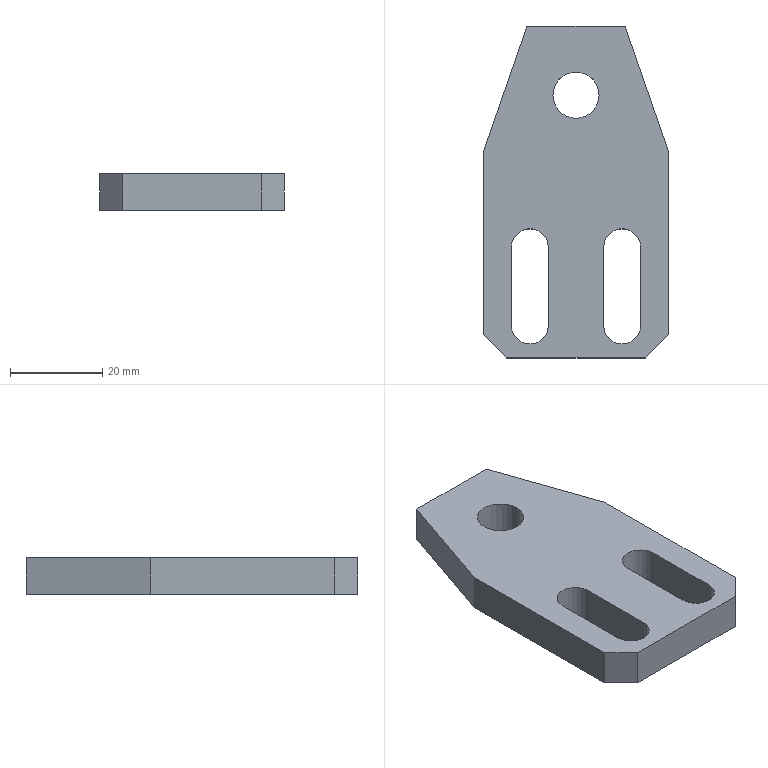Part | SolidWorks | features Chamfer 1, Extrusion 1 | 1 solid | 20 faces | box 40 x 72 x 8 mm | volume 17211 mm3 | plane 14 | cylinder 6 | commonest cylinder face diameters 8 x4 10 x2
STEP:
#1=CARTESIAN_POINT('',(-5.,57.,8.));
#2=VERTEX_POINT('',#1);
#3=CARTESIAN_POINT('',(5.,57.,8.));
#4=VERTEX_POINT('',#3);
#5=CARTESIAN_POINT('',(0.,57.,8.));
#6=DIRECTION('',(0.,0.,1.));
#7=DIRECTION('',(1.,0.,0.));
#8=AXIS2_PLACEMENT_3D('',#5,#6,#7);
#9=CIRCLE('',#8,5.);
#10=EDGE_CURVE('',#2,#4,#9,.T.);
#11=ORIENTED_EDGE('',*,*,#10,.T.);
#12=CARTESIAN_POINT('',(5.,57.,0.));
#13=VERTEX_POINT('',#12);
#14=CARTESIAN_POINT('',(5.,57.,8.));
#15=DIRECTION('',(0.,0.,-1.));
#16=VECTOR('',#15,1000.);
#17=LINE('',#14,#16);
#18=EDGE_CURVE('',#4,#13,#17,.T.);
#19=ORIENTED_EDGE('',*,*,#18,.T.);
#20=CARTESIAN_POINT('',(-5.,57.,0.));
#21=VERTEX_POINT('',#20);
#22=CARTESIAN_POINT('',(0.,57.,0.));
#23=DIRECTION('',(0.,0.,1.));
#24=DIRECTION('',(1.,0.,0.));
#25=AXIS2_PLACEMENT_3D('',#22,#23,#24);
#26=CIRCLE('',#25,5.);
#27=EDGE_CURVE('',#21,#13,#26,.T.);
#28=ORIENTED_EDGE('',*,*,#27,.F.);
#29=CARTESIAN_POINT('',(-5.,57.,8.));
#30=DIRECTION('',(0.,0.,-1.));
#31=VECTOR('',#30,1000.);
#32=LINE('',#29,#31);
#33=EDGE_CURVE('',#2,#21,#32,.T.);
#34=ORIENTED_EDGE('',*,*,#33,.F.);
#35=EDGE_LOOP('',(#11,#19,#28,#34));
#36=FACE_OUTER_BOUND('',#35,.T.);
#37=CARTESIAN_POINT('',(0.,57.,8.));
#38=DIRECTION('',(0.,0.,-1.));
#39=DIRECTION('',(-1.,0.,0.));
#40=AXIS2_PLACEMENT_3D('',#37,#38,#39);
#41=CYLINDRICAL_SURFACE('',#40,5.);
#42=ADVANCED_FACE('',(#36),#41,.F.);
#43=CARTESIAN_POINT('',(14.,7.,0.));
#44=VERTEX_POINT('',#43);
#45=CARTESIAN_POINT('',(14.,24.,0.));
#46=VERTEX_POINT('',#45);
#47=CARTESIAN_POINT('',(14.,0.,0.));
#48=DIRECTION('',(0.,1.,0.));
#49=VECTOR('',#48,1000.);
#50=LINE('',#47,#49);
#51=EDGE_CURVE('',#44,#46,#50,.T.);
#52=ORIENTED_EDGE('',*,*,#51,.F.);
#53=CARTESIAN_POINT('',(14.,7.,8.));
#54=VERTEX_POINT('',#53);
#55=CARTESIAN_POINT('',(14.,7.,8.));
#56=DIRECTION('',(0.,0.,-1.));
#57=VECTOR('',#56,1000.);
#58=LINE('',#55,#57);
#59=EDGE_CURVE('',#54,#44,#58,.T.);
#60=ORIENTED_EDGE('',*,*,#59,.F.);
#61=CARTESIAN_POINT('',(14.,24.,8.));
#62=VERTEX_POINT('',#61);
#63=CARTESIAN_POINT('',(14.,0.,8.));
#64=DIRECTION('',(0.,1.,0.));
#65=VECTOR('',#64,1000.);
#66=LINE('',#63,#65);
#67=EDGE_CURVE('',#54,#62,#66,.T.);
#68=ORIENTED_EDGE('',*,*,#67,.T.);
#69=CARTESIAN_POINT('',(14.,24.,8.));
#70=DIRECTION('',(0.,0.,-1.));
#71=VECTOR('',#70,1000.);
#72=LINE('',#69,#71);
#73=EDGE_CURVE('',#62,#46,#72,.T.);
#74=ORIENTED_EDGE('',*,*,#73,.T.);
#75=EDGE_LOOP('',(#52,#60,#68,#74));
#76=FACE_OUTER_BOUND('',#75,.T.);
#77=CARTESIAN_POINT('',(14.,0.,8.));
#78=DIRECTION('',(-1.,0.,0.));
#79=DIRECTION('',(0.,-1.,0.));
#80=AXIS2_PLACEMENT_3D('',#77,#78,#79);
#81=PLANE('',#80);
#82=ADVANCED_FACE('',(#76),#81,.T.);
#83=CARTESIAN_POINT('',(6.,7.,0.));
#84=VERTEX_POINT('',#83);
#85=CARTESIAN_POINT('',(10.,7.,0.));
#86=DIRECTION('',(0.,0.,-1.));
#87=DIRECTION('',(1.,0.,0.));
#88=AXIS2_PLACEMENT_3D('',#85,#86,#87);
#89=CIRCLE('',#88,4.);
#90=EDGE_CURVE('',#44,#84,#89,.T.);
#91=ORIENTED_EDGE('',*,*,#90,.T.);
#92=CARTESIAN_POINT('',(6.,7.,8.));
#93=VERTEX_POINT('',#92);
#94=CARTESIAN_POINT('',(6.,7.,8.));
#95=DIRECTION('',(0.,0.,-1.));
#96=VECTOR('',#95,1000.);
#97=LINE('',#94,#96);
#98=EDGE_CURVE('',#93,#84,#97,.T.);
#99=ORIENTED_EDGE('',*,*,#98,.F.);
#100=CARTESIAN_POINT('',(10.,7.,8.));
#101=DIRECTION('',(0.,0.,-1.));
#102=DIRECTION('',(1.,0.,0.));
#103=AXIS2_PLACEMENT_3D('',#100,#101,#102);
#104=CIRCLE('',#103,4.);
#105=EDGE_CURVE('',#54,#93,#104,.T.);
#106=ORIENTED_EDGE('',*,*,#105,.F.);
#107=ORIENTED_EDGE('',*,*,#59,.T.);
#108=EDGE_LOOP('',(#91,#99,#106,#107));
#109=FACE_OUTER_BOUND('',#108,.T.);
#110=CARTESIAN_POINT('',(10.,7.,8.));
#111=DIRECTION('',(0.,0.,-1.));
#112=DIRECTION('',(-1.,0.,0.));
#113=AXIS2_PLACEMENT_3D('',#110,#111,#112);
#114=CYLINDRICAL_SURFACE('',#113,4.);
#115=ADVANCED_FACE('',(#109),#114,.F.);
#116=CARTESIAN_POINT('',(6.,24.,0.));
#117=VERTEX_POINT('',#116);
#118=CARTESIAN_POINT('',(6.,0.,0.));
#119=DIRECTION('',(0.,1.,0.));
#120=VECTOR('',#119,1000.);
#121=LINE('',#118,#120);
#122=EDGE_CURVE('',#84,#117,#121,.T.);
#123=ORIENTED_EDGE('',*,*,#122,.T.);
#124=CARTESIAN_POINT('',(6.,24.,8.));
#125=VERTEX_POINT('',#124);
#126=CARTESIAN_POINT('',(6.,24.,8.));
#127=DIRECTION('',(0.,0.,-1.));
#128=VECTOR('',#127,1000.);
#129=LINE('',#126,#128);
#130=EDGE_CURVE('',#125,#117,#129,.T.);
#131=ORIENTED_EDGE('',*,*,#130,.F.);
#132=CARTESIAN_POINT('',(6.,0.,8.));
#133=DIRECTION('',(0.,1.,0.));
#134=VECTOR('',#133,1000.);
#135=LINE('',#132,#134);
#136=EDGE_CURVE('',#93,#125,#135,.T.);
#137=ORIENTED_EDGE('',*,*,#136,.F.);
#138=ORIENTED_EDGE('',*,*,#98,.T.);
#139=EDGE_LOOP('',(#123,#131,#137,#138));
#140=FACE_OUTER_BOUND('',#139,.T.);
#141=CARTESIAN_POINT('',(6.,0.,8.));
#142=DIRECTION('',(-1.,0.,0.));
#143=DIRECTION('',(0.,0.,1.));
#144=AXIS2_PLACEMENT_3D('',#141,#142,#143);
#145=PLANE('',#144);
#146=ADVANCED_FACE('',(#140),#145,.F.);
#147=CARTESIAN_POINT('',(-15.,0.,8.));
#148=VERTEX_POINT('',#147);
#149=CARTESIAN_POINT('',(15.,0.,8.));
#150=VERTEX_POINT('',#149);
#151=CARTESIAN_POINT('',(0.,0.,8.));
#152=DIRECTION('',(1.,0.,0.));
#153=VECTOR('',#152,1000.);
#154=LINE('',#151,#153);
#155=EDGE_CURVE('',#148,#150,#154,.T.);
#156=ORIENTED_EDGE('',*,*,#155,.F.);
#157=CARTESIAN_POINT('',(-15.,0.,0.));
#158=VERTEX_POINT('',#157);
#159=CARTESIAN_POINT('',(-15.,0.,8.));
#160=DIRECTION('',(0.,0.,-1.));
#161=VECTOR('',#160,1000.);
#162=LINE('',#159,#161);
#163=EDGE_CURVE('',#148,#158,#162,.T.);
#164=ORIENTED_EDGE('',*,*,#163,.T.);
#165=CARTESIAN_POINT('',(15.,0.,0.));
#166=VERTEX_POINT('',#165);
#167=CARTESIAN_POINT('',(0.,0.,0.));
#168=DIRECTION('',(1.,0.,0.));
#169=VECTOR('',#168,1000.);
#170=LINE('',#167,#169);
#171=EDGE_CURVE('',#158,#166,#170,.T.);
#172=ORIENTED_EDGE('',*,*,#171,.T.);
#173=CARTESIAN_POINT('',(15.,0.,8.));
#174=DIRECTION('',(0.,0.,1.));
#175=VECTOR('',#174,1000.);
#176=LINE('',#173,#175);
#177=EDGE_CURVE('',#166,#150,#176,.T.);
#178=ORIENTED_EDGE('',*,*,#177,.T.);
#179=EDGE_LOOP('',(#156,#164,#172,#178));
#180=FACE_OUTER_BOUND('',#179,.T.);
#181=CARTESIAN_POINT('',(0.,0.,8.));
#182=DIRECTION('',(0.,1.,0.));
#183=DIRECTION('',(0.,0.,1.));
#184=AXIS2_PLACEMENT_3D('',#181,#182,#183);
#185=PLANE('',#184);
#186=ADVANCED_FACE('',(#180),#185,.F.);
#187=CARTESIAN_POINT('',(20.,5.,8.));
#188=VERTEX_POINT('',#187);
#189=CARTESIAN_POINT('',(20.,45.,8.));
#190=VERTEX_POINT('',#189);
#191=CARTESIAN_POINT('',(20.,0.,8.));
#192=DIRECTION('',(0.,1.,0.));
#193=VECTOR('',#192,1000.);
#194=LINE('',#191,#193);
#195=EDGE_CURVE('',#188,#190,#194,.T.);
#196=ORIENTED_EDGE('',*,*,#195,.F.);
#197=CARTESIAN_POINT('',(20.,5.,0.));
#198=VERTEX_POINT('',#197);
#199=CARTESIAN_POINT('',(20.,5.,8.));
#200=DIRECTION('',(0.,0.,-1.));
#201=VECTOR('',#200,1000.);
#202=LINE('',#199,#201);
#203=EDGE_CURVE('',#188,#198,#202,.T.);
#204=ORIENTED_EDGE('',*,*,#203,.T.);
#205=CARTESIAN_POINT('',(20.,45.,0.));
#206=VERTEX_POINT('',#205);
#207=CARTESIAN_POINT('',(20.,0.,0.));
#208=DIRECTION('',(0.,1.,0.));
#209=VECTOR('',#208,1000.);
#210=LINE('',#207,#209);
#211=EDGE_CURVE('',#198,#206,#210,.T.);
#212=ORIENTED_EDGE('',*,*,#211,.T.);
#213=CARTESIAN_POINT('',(20.,45.,8.));
#214=DIRECTION('',(0.,0.,-1.));
#215=VECTOR('',#214,1000.);
#216=LINE('',#213,#215);
#217=EDGE_CURVE('',#190,#206,#216,.T.);
#218=ORIENTED_EDGE('',*,*,#217,.F.);
#219=EDGE_LOOP('',(#196,#204,#212,#218));
#220=FACE_OUTER_BOUND('',#219,.T.);
#221=CARTESIAN_POINT('',(20.,0.,8.));
#222=DIRECTION('',(-1.,0.,0.));
#223=DIRECTION('',(0.,-1.,0.));
#224=AXIS2_PLACEMENT_3D('',#221,#222,#223);
#225=PLANE('',#224);
#226=ADVANCED_FACE('',(#220),#225,.F.);
#227=CARTESIAN_POINT('',(10.645,72.,0.));
#228=VERTEX_POINT('',#227);
#229=CARTESIAN_POINT('',(31.777,11.01,0.));
#230=DIRECTION('',(-0.3274,0.9449,0.));
#231=VECTOR('',#230,1000.);
#232=LINE('',#229,#231);
#233=EDGE_CURVE('',#206,#228,#232,.T.);
#234=ORIENTED_EDGE('',*,*,#233,.T.);
#235=CARTESIAN_POINT('',(10.645,72.,8.));
#236=VERTEX_POINT('',#235);
#237=CARTESIAN_POINT('',(10.645,72.,8.));
#238=DIRECTION('',(0.,0.,-1.));
#239=VECTOR('',#238,1000.);
#240=LINE('',#237,#239);
#241=EDGE_CURVE('',#236,#228,#240,.T.);
#242=ORIENTED_EDGE('',*,*,#241,.F.);
#243=CARTESIAN_POINT('',(31.777,11.01,8.));
#244=DIRECTION('',(-0.3274,0.9449,0.));
#245=VECTOR('',#244,1000.);
#246=LINE('',#243,#245);
#247=EDGE_CURVE('',#190,#236,#246,.T.);
#248=ORIENTED_EDGE('',*,*,#247,.F.);
#249=ORIENTED_EDGE('',*,*,#217,.T.);
#250=EDGE_LOOP('',(#234,#242,#248,#249));
#251=FACE_OUTER_BOUND('',#250,.T.);
#252=CARTESIAN_POINT('',(31.777,11.01,8.));
#253=DIRECTION('',(-0.9449,-0.3274,0.));
#254=DIRECTION('',(0.3274,-0.9449,0.));
#255=AXIS2_PLACEMENT_3D('',#252,#253,#254);
#256=PLANE('',#255);
#257=ADVANCED_FACE('',(#251),#256,.F.);
#258=CARTESIAN_POINT('',(-10.645,72.,0.));
#259=VERTEX_POINT('',#258);
#260=CARTESIAN_POINT('',(0.,72.,0.));
#261=DIRECTION('',(-1.,0.,0.));
#262=VECTOR('',#261,1000.);
#263=LINE('',#260,#262);
#264=EDGE_CURVE('',#228,#259,#263,.T.);
#265=ORIENTED_EDGE('',*,*,#264,.T.);
#266=CARTESIAN_POINT('',(-10.645,72.,8.));
#267=VERTEX_POINT('',#266);
#268=CARTESIAN_POINT('',(-10.645,72.,8.));
#269=DIRECTION('',(0.,0.,-1.));
#270=VECTOR('',#269,1000.);
#271=LINE('',#268,#270);
#272=EDGE_CURVE('',#267,#259,#271,.T.);
#273=ORIENTED_EDGE('',*,*,#272,.F.);
#274=CARTESIAN_POINT('',(0.,72.,8.));
#275=DIRECTION('',(-1.,0.,0.));
#276=VECTOR('',#275,1000.);
#277=LINE('',#274,#276);
#278=EDGE_CURVE('',#236,#267,#277,.T.);
#279=ORIENTED_EDGE('',*,*,#278,.F.);
#280=ORIENTED_EDGE('',*,*,#241,.T.);
#281=EDGE_LOOP('',(#265,#273,#279,#280));
#282=FACE_OUTER_BOUND('',#281,.T.);
#283=CARTESIAN_POINT('',(0.,72.,8.));
#284=DIRECTION('',(0.,-1.,0.));
#285=DIRECTION('',(0.,0.,-1.));
#286=AXIS2_PLACEMENT_3D('',#283,#284,#285);
#287=PLANE('',#286);
#288=ADVANCED_FACE('',(#282),#287,.F.);
#289=CARTESIAN_POINT('',(-20.,45.,0.));
#290=VERTEX_POINT('',#289);
#291=CARTESIAN_POINT('',(-31.777,11.01,0.));
#292=DIRECTION('',(-0.3274,-0.9449,0.));
#293=VECTOR('',#292,1000.);
#294=LINE('',#291,#293);
#295=EDGE_CURVE('',#259,#290,#294,.T.);
#296=ORIENTED_EDGE('',*,*,#295,.T.);
#297=CARTESIAN_POINT('',(-20.,45.,8.));
#298=VERTEX_POINT('',#297);
#299=CARTESIAN_POINT('',(-20.,45.,8.));
#300=DIRECTION('',(0.,0.,-1.));
#301=VECTOR('',#300,1000.);
#302=LINE('',#299,#301);
#303=EDGE_CURVE('',#298,#290,#302,.T.);
#304=ORIENTED_EDGE('',*,*,#303,.F.);
#305=CARTESIAN_POINT('',(-31.777,11.01,8.));
#306=DIRECTION('',(-0.3274,-0.9449,0.));
#307=VECTOR('',#306,1000.);
#308=LINE('',#305,#307);
#309=EDGE_CURVE('',#267,#298,#308,.T.);
#310=ORIENTED_EDGE('',*,*,#309,.F.);
#311=ORIENTED_EDGE('',*,*,#272,.T.);
#312=EDGE_LOOP('',(#296,#304,#310,#311));
#313=FACE_OUTER_BOUND('',#312,.T.);
#314=CARTESIAN_POINT('',(-31.777,11.01,8.));
#315=DIRECTION('',(0.9449,-0.3274,0.));
#316=DIRECTION('',(0.3274,0.9449,0.));
#317=AXIS2_PLACEMENT_3D('',#314,#315,#316);
#318=PLANE('',#317);
#319=ADVANCED_FACE('',(#313),#318,.F.);
#320=CARTESIAN_POINT('',(-6.,24.,0.));
#321=VERTEX_POINT('',#320);
#322=CARTESIAN_POINT('',(-14.,24.,0.));
#323=VERTEX_POINT('',#322);
#324=CARTESIAN_POINT('',(-10.,24.,0.));
#325=DIRECTION('',(0.,0.,1.));
#326=DIRECTION('',(1.,0.,0.));
#327=AXIS2_PLACEMENT_3D('',#324,#325,#326);
#328=CIRCLE('',#327,4.);
#329=EDGE_CURVE('',#321,#323,#328,.T.);
#330=ORIENTED_EDGE('',*,*,#329,.F.);
#331=CARTESIAN_POINT('',(-6.,24.,8.));
#332=VERTEX_POINT('',#331);
#333=CARTESIAN_POINT('',(-6.,24.,8.));
#334=DIRECTION('',(0.,0.,-1.));
#335=VECTOR('',#334,1000.);
#336=LINE('',#333,#335);
#337=EDGE_CURVE('',#332,#321,#336,.T.);
#338=ORIENTED_EDGE('',*,*,#337,.F.);
#339=CARTESIAN_POINT('',(-14.,24.,8.));
#340=VERTEX_POINT('',#339);
#341=CARTESIAN_POINT('',(-10.,24.,8.));
#342=DIRECTION('',(0.,0.,1.));
#343=DIRECTION('',(1.,0.,0.));
#344=AXIS2_PLACEMENT_3D('',#341,#342,#343);
#345=CIRCLE('',#344,4.);
#346=EDGE_CURVE('',#332,#340,#345,.T.);
#347=ORIENTED_EDGE('',*,*,#346,.T.);
#348=CARTESIAN_POINT('',(-14.,24.,8.));
#349=DIRECTION('',(0.,0.,-1.));
#350=VECTOR('',#349,1000.);
#351=LINE('',#348,#350);
#352=EDGE_CURVE('',#340,#323,#351,.T.);
#353=ORIENTED_EDGE('',*,*,#352,.T.);
#354=EDGE_LOOP('',(#330,#338,#347,#353));
#355=FACE_OUTER_BOUND('',#354,.T.);
#356=CARTESIAN_POINT('',(-10.,24.,8.));
#357=DIRECTION('',(0.,0.,-1.));
#358=DIRECTION('',(-1.,0.,0.));
#359=AXIS2_PLACEMENT_3D('',#356,#357,#358);
#360=CYLINDRICAL_SURFACE('',#359,4.);
#361=ADVANCED_FACE('',(#355),#360,.F.);
#362=CARTESIAN_POINT('',(-6.,7.,0.));
#363=VERTEX_POINT('',#362);
#364=CARTESIAN_POINT('',(-6.,0.,0.));
#365=DIRECTION('',(0.,1.,0.));
#366=VECTOR('',#365,1000.);
#367=LINE('',#364,#366);
#368=EDGE_CURVE('',#363,#321,#367,.T.);
#369=ORIENTED_EDGE('',*,*,#368,.F.);
#370=CARTESIAN_POINT('',(-6.,7.,8.));
#371=VERTEX_POINT('',#370);
#372=CARTESIAN_POINT('',(-6.,7.,8.));
#373=DIRECTION('',(0.,0.,-1.));
#374=VECTOR('',#373,1000.);
#375=LINE('',#372,#374);
#376=EDGE_CURVE('',#371,#363,#375,.T.);
#377=ORIENTED_EDGE('',*,*,#376,.F.);
#378=CARTESIAN_POINT('',(-6.,0.,8.));
#379=DIRECTION('',(0.,1.,0.));
#380=VECTOR('',#379,1000.);
#381=LINE('',#378,#380);
#382=EDGE_CURVE('',#371,#332,#381,.T.);
#383=ORIENTED_EDGE('',*,*,#382,.T.);
#384=ORIENTED_EDGE('',*,*,#337,.T.);
#385=EDGE_LOOP('',(#369,#377,#383,#384));
#386=FACE_OUTER_BOUND('',#385,.T.);
#387=CARTESIAN_POINT('',(-6.,0.,8.));
#388=DIRECTION('',(-1.,0.,0.));
#389=DIRECTION('',(0.,0.,1.));
#390=AXIS2_PLACEMENT_3D('',#387,#388,#389);
#391=PLANE('',#390);
#392=ADVANCED_FACE('',(#386),#391,.T.);
#393=CARTESIAN_POINT('',(-14.,7.,0.));
#394=VERTEX_POINT('',#393);
#395=CARTESIAN_POINT('',(-10.,7.,0.));
#396=DIRECTION('',(0.,0.,1.));
#397=DIRECTION('',(1.,0.,0.));
#398=AXIS2_PLACEMENT_3D('',#395,#396,#397);
#399=CIRCLE('',#398,4.);
#400=EDGE_CURVE('',#394,#363,#399,.T.);
#401=ORIENTED_EDGE('',*,*,#400,.F.);
#402=CARTESIAN_POINT('',(-14.,7.,8.));
#403=VERTEX_POINT('',#402);
#404=CARTESIAN_POINT('',(-14.,7.,8.));
#405=DIRECTION('',(0.,0.,-1.));
#406=VECTOR('',#405,1000.);
#407=LINE('',#404,#406);
#408=EDGE_CURVE('',#403,#394,#407,.T.);
#409=ORIENTED_EDGE('',*,*,#408,.F.);
#410=CARTESIAN_POINT('',(-10.,7.,8.));
#411=DIRECTION('',(0.,0.,1.));
#412=DIRECTION('',(1.,0.,0.));
#413=AXIS2_PLACEMENT_3D('',#410,#411,#412);
#414=CIRCLE('',#413,4.);
#415=EDGE_CURVE('',#403,#371,#414,.T.);
#416=ORIENTED_EDGE('',*,*,#415,.T.);
#417=ORIENTED_EDGE('',*,*,#376,.T.);
#418=EDGE_LOOP('',(#401,#409,#416,#417));
#419=FACE_OUTER_BOUND('',#418,.T.);
#420=CARTESIAN_POINT('',(-10.,7.,8.));
#421=DIRECTION('',(0.,0.,-1.));
#422=DIRECTION('',(-1.,0.,0.));
#423=AXIS2_PLACEMENT_3D('',#420,#421,#422);
#424=CYLINDRICAL_SURFACE('',#423,4.);
#425=ADVANCED_FACE('',(#419),#424,.F.);
#426=CARTESIAN_POINT('',(-20.,5.,0.));
#427=VERTEX_POINT('',#426);
#428=CARTESIAN_POINT('',(-20.,0.,0.));
#429=DIRECTION('',(0.,-1.,0.));
#430=VECTOR('',#429,1000.);
#431=LINE('',#428,#430);
#432=EDGE_CURVE('',#290,#427,#431,.T.);
#433=ORIENTED_EDGE('',*,*,#432,.T.);
#434=CARTESIAN_POINT('',(-20.,5.,8.));
#435=VERTEX_POINT('',#434);
#436=CARTESIAN_POINT('',(-20.,5.,8.));
#437=DIRECTION('',(0.,0.,1.));
#438=VECTOR('',#437,1000.);
#439=LINE('',#436,#438);
#440=EDGE_CURVE('',#427,#435,#439,.T.);
#441=ORIENTED_EDGE('',*,*,#440,.T.);
#442=CARTESIAN_POINT('',(-20.,0.,8.));
#443=DIRECTION('',(0.,-1.,0.));
#444=VECTOR('',#443,1000.);
#445=LINE('',#442,#444);
#446=EDGE_CURVE('',#298,#435,#445,.T.);
#447=ORIENTED_EDGE('',*,*,#446,.F.);
#448=ORIENTED_EDGE('',*,*,#303,.T.);
#449=EDGE_LOOP('',(#433,#441,#447,#448));
#450=FACE_OUTER_BOUND('',#449,.T.);
#451=CARTESIAN_POINT('',(-20.,0.,8.));
#452=DIRECTION('',(1.,0.,0.));
#453=DIRECTION('',(0.,0.,-1.));
#454=AXIS2_PLACEMENT_3D('',#451,#452,#453);
#455=PLANE('',#454);
#456=ADVANCED_FACE('',(#450),#455,.F.);
#457=CARTESIAN_POINT('',(-14.,0.,0.));
#458=DIRECTION('',(0.,1.,0.));
#459=VECTOR('',#458,1000.);
#460=LINE('',#457,#459);
#461=EDGE_CURVE('',#394,#323,#460,.T.);
#462=ORIENTED_EDGE('',*,*,#461,.T.);
#463=ORIENTED_EDGE('',*,*,#352,.F.);
#464=CARTESIAN_POINT('',(-14.,0.,8.));
#465=DIRECTION('',(0.,1.,0.));
#466=VECTOR('',#465,1000.);
#467=LINE('',#464,#466);
#468=EDGE_CURVE('',#403,#340,#467,.T.);
#469=ORIENTED_EDGE('',*,*,#468,.F.);
#470=ORIENTED_EDGE('',*,*,#408,.T.);
#471=EDGE_LOOP('',(#462,#463,#469,#470));
#472=FACE_OUTER_BOUND('',#471,.T.);
#473=CARTESIAN_POINT('',(-14.,0.,8.));
#474=DIRECTION('',(-1.,0.,0.));
#475=DIRECTION('',(0.,0.,1.));
#476=AXIS2_PLACEMENT_3D('',#473,#474,#475);
#477=PLANE('',#476);
#478=ADVANCED_FACE('',(#472),#477,.F.);
#479=ORIENTED_EDGE('',*,*,#18,.F.);
#480=CARTESIAN_POINT('',(0.,57.,8.));
#481=DIRECTION('',(0.,0.,1.));
#482=DIRECTION('',(1.,0.,0.));
#483=AXIS2_PLACEMENT_3D('',#480,#481,#482);
#484=CIRCLE('',#483,5.);
#485=EDGE_CURVE('',#4,#2,#484,.T.);
#486=ORIENTED_EDGE('',*,*,#485,.T.);
#487=ORIENTED_EDGE('',*,*,#33,.T.);
#488=CARTESIAN_POINT('',(0.,57.,0.));
#489=DIRECTION('',(0.,0.,1.));
#490=DIRECTION('',(1.,0.,0.));
#491=AXIS2_PLACEMENT_3D('',#488,#489,#490);
#492=CIRCLE('',#491,5.);
#493=EDGE_CURVE('',#13,#21,#492,.T.);
#494=ORIENTED_EDGE('',*,*,#493,.F.);
#495=EDGE_LOOP('',(#479,#486,#487,#494));
#496=FACE_OUTER_BOUND('',#495,.T.);
#497=CARTESIAN_POINT('',(0.,57.,8.));
#498=DIRECTION('',(0.,0.,-1.));
#499=DIRECTION('',(-1.,0.,0.));
#500=AXIS2_PLACEMENT_3D('',#497,#498,#499);
#501=CYLINDRICAL_SURFACE('',#500,5.);
#502=ADVANCED_FACE('',(#496),#501,.F.);
#503=CARTESIAN_POINT('',(10.,24.,0.));
#504=DIRECTION('',(0.,0.,-1.));
#505=DIRECTION('',(1.,0.,0.));
#506=AXIS2_PLACEMENT_3D('',#503,#504,#505);
#507=CIRCLE('',#506,4.);
#508=EDGE_CURVE('',#117,#46,#507,.T.);
#509=ORIENTED_EDGE('',*,*,#508,.T.);
#510=ORIENTED_EDGE('',*,*,#73,.F.);
#511=CARTESIAN_POINT('',(10.,24.,8.));
#512=DIRECTION('',(0.,0.,-1.));
#513=DIRECTION('',(1.,0.,0.));
#514=AXIS2_PLACEMENT_3D('',#511,#512,#513);
#515=CIRCLE('',#514,4.);
#516=EDGE_CURVE('',#125,#62,#515,.T.);
#517=ORIENTED_EDGE('',*,*,#516,.F.);
#518=ORIENTED_EDGE('',*,*,#130,.T.);
#519=EDGE_LOOP('',(#509,#510,#517,#518));
#520=FACE_OUTER_BOUND('',#519,.T.);
#521=CARTESIAN_POINT('',(10.,24.,8.));
#522=DIRECTION('',(0.,0.,-1.));
#523=DIRECTION('',(-1.,0.,0.));
#524=AXIS2_PLACEMENT_3D('',#521,#522,#523);
#525=CYLINDRICAL_SURFACE('',#524,4.);
#526=ADVANCED_FACE('',(#520),#525,.F.);
#527=ORIENTED_EDGE('',*,*,#10,.F.);
#528=ORIENTED_EDGE('',*,*,#485,.F.);
#529=EDGE_LOOP('',(#527,#528));
#530=FACE_BOUND('',#529,.T.);
#531=ORIENTED_EDGE('',*,*,#346,.F.);
#532=ORIENTED_EDGE('',*,*,#382,.F.);
#533=ORIENTED_EDGE('',*,*,#415,.F.);
#534=ORIENTED_EDGE('',*,*,#468,.T.);
#535=EDGE_LOOP('',(#531,#532,#533,#534));
#536=FACE_BOUND('',#535,.T.);
#537=ORIENTED_EDGE('',*,*,#446,.T.);
#538=CARTESIAN_POINT('',(-7.5,-7.5,8.));
#539=DIRECTION('',(0.7071,-0.7071,0.));
#540=VECTOR('',#539,1000.);
#541=LINE('',#538,#540);
#542=EDGE_CURVE('',#435,#148,#541,.T.);
#543=ORIENTED_EDGE('',*,*,#542,.T.);
#544=ORIENTED_EDGE('',*,*,#155,.T.);
#545=CARTESIAN_POINT('',(7.5,-7.5,8.));
#546=DIRECTION('',(0.7071,0.7071,0.));
#547=VECTOR('',#546,1000.);
#548=LINE('',#545,#547);
#549=EDGE_CURVE('',#150,#188,#548,.T.);
#550=ORIENTED_EDGE('',*,*,#549,.T.);
#551=ORIENTED_EDGE('',*,*,#195,.T.);
#552=ORIENTED_EDGE('',*,*,#247,.T.);
#553=ORIENTED_EDGE('',*,*,#278,.T.);
#554=ORIENTED_EDGE('',*,*,#309,.T.);
#555=EDGE_LOOP('',(#537,#543,#544,#550,#551,#552,#553,#554));
#556=FACE_OUTER_BOUND('',#555,.T.);
#557=ORIENTED_EDGE('',*,*,#67,.F.);
#558=ORIENTED_EDGE('',*,*,#105,.T.);
#559=ORIENTED_EDGE('',*,*,#136,.T.);
#560=ORIENTED_EDGE('',*,*,#516,.T.);
#561=EDGE_LOOP('',(#557,#558,#559,#560));
#562=FACE_BOUND('',#561,.T.);
#563=CARTESIAN_POINT('',(0.,0.,8.));
#564=DIRECTION('',(0.,0.,1.));
#565=DIRECTION('',(1.,0.,0.));
#566=AXIS2_PLACEMENT_3D('',#563,#564,#565);
#567=PLANE('',#566);
#568=ADVANCED_FACE('',(#530,#536,#556,#562),#567,.T.);
#569=ORIENTED_EDGE('',*,*,#27,.T.);
#570=ORIENTED_EDGE('',*,*,#493,.T.);
#571=EDGE_LOOP('',(#569,#570));
#572=FACE_BOUND('',#571,.T.);
#573=ORIENTED_EDGE('',*,*,#329,.T.);
#574=ORIENTED_EDGE('',*,*,#461,.F.);
#575=ORIENTED_EDGE('',*,*,#400,.T.);
#576=ORIENTED_EDGE('',*,*,#368,.T.);
#577=EDGE_LOOP('',(#573,#574,#575,#576));
#578=FACE_BOUND('',#577,.T.);
#579=ORIENTED_EDGE('',*,*,#171,.F.);
#580=CARTESIAN_POINT('',(-15.,0.,0.));
#581=DIRECTION('',(-0.7071,0.7071,0.));
#582=VECTOR('',#581,1000.);
#583=LINE('',#580,#582);
#584=EDGE_CURVE('',#158,#427,#583,.T.);
#585=ORIENTED_EDGE('',*,*,#584,.T.);
#586=ORIENTED_EDGE('',*,*,#432,.F.);
#587=ORIENTED_EDGE('',*,*,#295,.F.);
#588=ORIENTED_EDGE('',*,*,#264,.F.);
#589=ORIENTED_EDGE('',*,*,#233,.F.);
#590=ORIENTED_EDGE('',*,*,#211,.F.);
#591=CARTESIAN_POINT('',(20.,5.,0.));
#592=DIRECTION('',(-0.7071,-0.7071,0.));
#593=VECTOR('',#592,1000.);
#594=LINE('',#591,#593);
#595=EDGE_CURVE('',#198,#166,#594,.T.);
#596=ORIENTED_EDGE('',*,*,#595,.T.);
#597=EDGE_LOOP('',(#579,#585,#586,#587,#588,#589,#590,#596));
#598=FACE_OUTER_BOUND('',#597,.T.);
#599=ORIENTED_EDGE('',*,*,#51,.T.);
#600=ORIENTED_EDGE('',*,*,#508,.F.);
#601=ORIENTED_EDGE('',*,*,#122,.F.);
#602=ORIENTED_EDGE('',*,*,#90,.F.);
#603=EDGE_LOOP('',(#599,#600,#601,#602));
#604=FACE_BOUND('',#603,.T.);
#605=CARTESIAN_POINT('',(0.,0.,0.));
#606=DIRECTION('',(0.,0.,1.));
#607=DIRECTION('',(1.,0.,0.));
#608=AXIS2_PLACEMENT_3D('',#605,#606,#607);
#609=PLANE('',#608);
#610=ADVANCED_FACE('',(#572,#578,#598,#604),#609,.F.);
#611=ORIENTED_EDGE('',*,*,#542,.F.);
#612=ORIENTED_EDGE('',*,*,#440,.F.);
#613=ORIENTED_EDGE('',*,*,#584,.F.);
#614=ORIENTED_EDGE('',*,*,#163,.F.);
#615=EDGE_LOOP('',(#611,#612,#613,#614));
#616=FACE_OUTER_BOUND('',#615,.T.);
#617=CARTESIAN_POINT('',(-15.,0.,8.));
#618=DIRECTION('',(0.7071,0.7071,0.));
#619=DIRECTION('',(0.,0.,-1.));
#620=AXIS2_PLACEMENT_3D('',#617,#618,#619);
#621=PLANE('',#620);
#622=ADVANCED_FACE('',(#616),#621,.F.);
#623=ORIENTED_EDGE('',*,*,#549,.F.);
#624=ORIENTED_EDGE('',*,*,#177,.F.);
#625=ORIENTED_EDGE('',*,*,#595,.F.);
#626=ORIENTED_EDGE('',*,*,#203,.F.);
#627=EDGE_LOOP('',(#623,#624,#625,#626));
#628=FACE_OUTER_BOUND('',#627,.T.);
#629=CARTESIAN_POINT('',(20.,5.,8.));
#630=DIRECTION('',(-0.7071,0.7071,0.));
#631=DIRECTION('',(0.,0.,-1.));
#632=AXIS2_PLACEMENT_3D('',#629,#630,#631);
#633=PLANE('',#632);
#634=ADVANCED_FACE('',(#628),#633,.F.);
#635=CLOSED_SHELL('',(#42,#82,#115,#146,#186,#226,#257,#288,#319,#361,#392,#425,#456,#478,#502,#526,#568,#610,#622,#634));
#636=MANIFOLD_SOLID_BREP('',#635);
#637=CARTESIAN_POINT('',(0.,0.,0.));
#638=DIRECTION('',(0.,0.,1.));
#639=DIRECTION('',(1.,0.,0.));
#640=AXIS2_PLACEMENT_3D('',#637,#638,#639);
#641=(LENGTH_UNIT()NAMED_UNIT(*)SI_UNIT(.MILLI.,.METRE.));
#642=UNCERTAINTY_MEASURE_WITH_UNIT(LENGTH_MEASURE(0.00001),#641,'','');
#643=(NAMED_UNIT(*)PLANE_ANGLE_UNIT()SI_UNIT($,.RADIAN.));
#644=(NAMED_UNIT(*)SI_UNIT($,.STERADIAN.)SOLID_ANGLE_UNIT());
#645=(GEOMETRIC_REPRESENTATION_CONTEXT(3)GLOBAL_UNCERTAINTY_ASSIGNED_CONTEXT((#642))GLOBAL_UNIT_ASSIGNED_CONTEXT((#641,#643,#644))REPRESENTATION_CONTEXT('',''));
#646=ADVANCED_BREP_SHAPE_REPRESENTATION('',(#636,#640),#645);